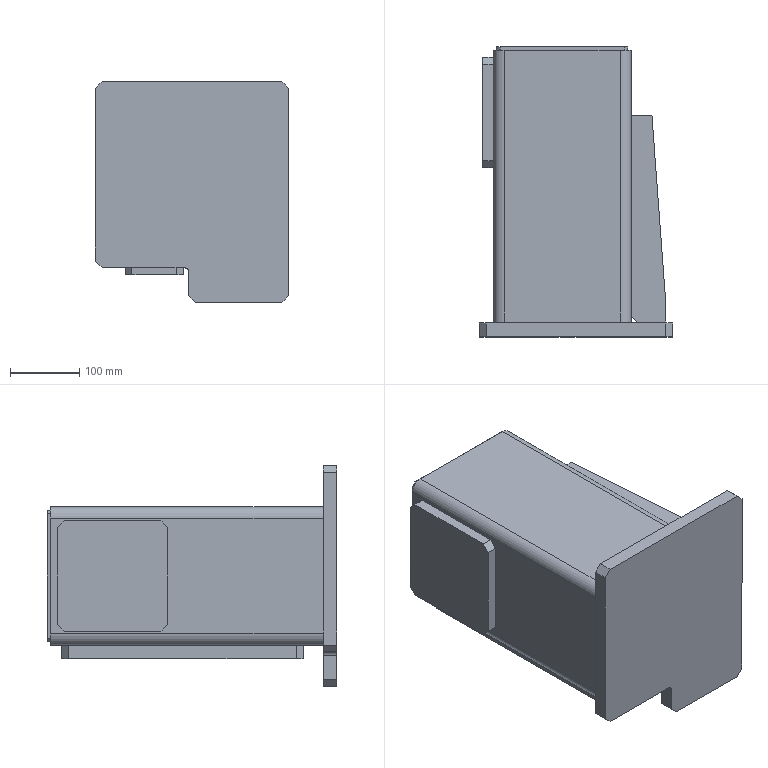Part | SolidWorks | features ICE 5, Chamfer 2, Extrusion 1, Fillet 1, MirrorPattern 1 | 1 solid | 72 faces | box 280 x 420 x 320 mm | volume 5533636 mm3 | plane 63 | cylinder 9 | commonest cylinder face diameters 16 x4 32 x4 10 x1